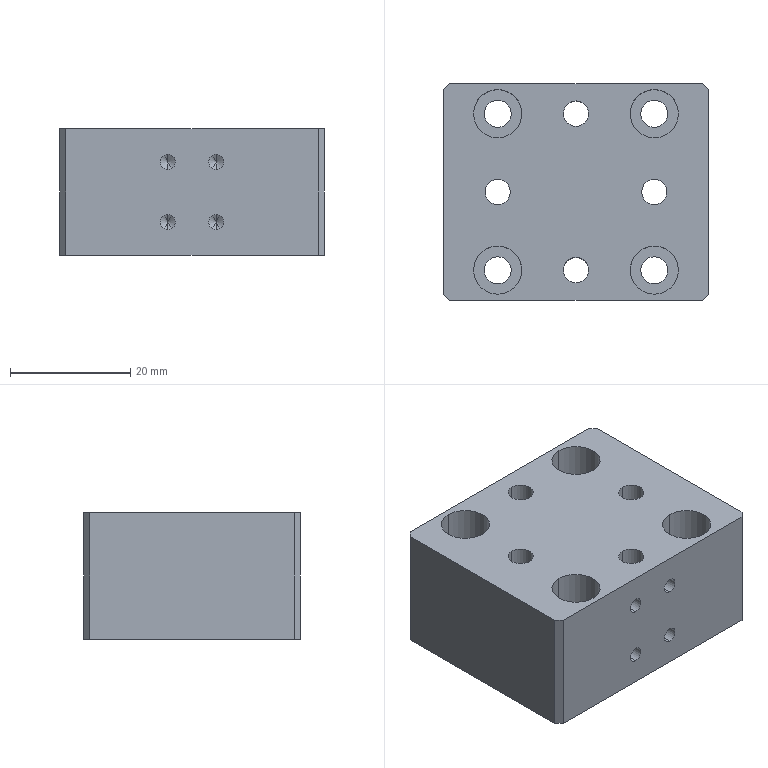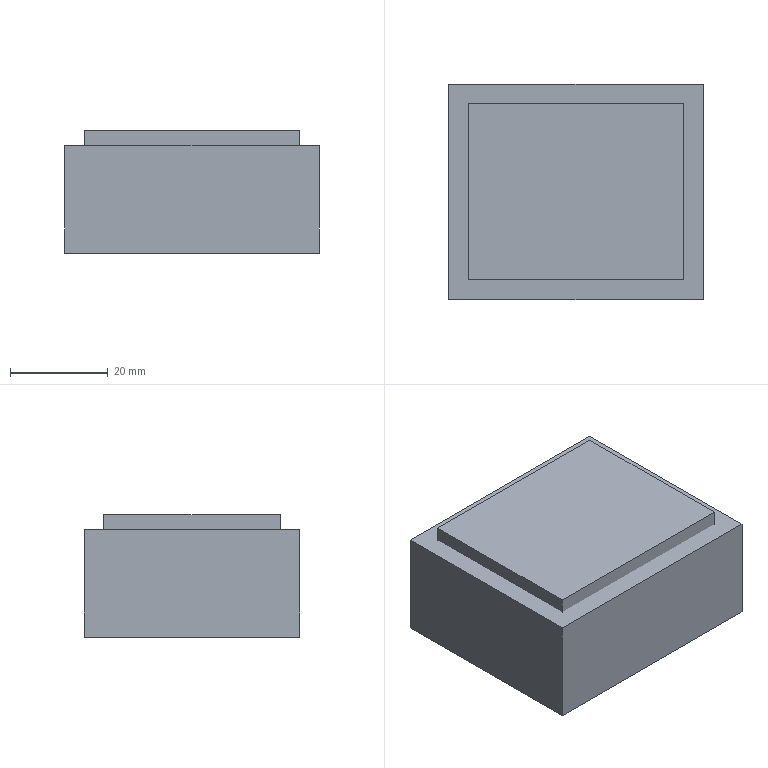CAM job | NX | 3+2 milling, drilling | part box 44 x 36 x 21 mm | stock box 52 x 44 x 25 mm
Tools:
number,name,description,diameter,corner_radius,flute_length,length,flutes
1,D63,Milling Tool-5 Parameters,63.0,0.0,50.0,75.0,2
7,D6A45,Milling Tool-5 Parameters,6.0,0.0,3.0,3.0,2
14,4.2ZT,Drilling Tool,4.2,0.0,35.0,50.0,2
15,M5,Milling Tool-5 Parameters,4.2,0.0,30.0,30.0,4
16,4.5ZT,Drilling Tool,4.5,0.0,35.0,50.0,2
4,D4,Milling Tool-5 Parameters,4.0,0.0,50.0,75.0,2
10,D10,Milling Tool-5 Parameters,10.0,0.0,50.0,75.0,2
11,D10JING,Milling Tool-5 Parameters,10.0,0.0,50.0,75.0,2
12,2.5ZT,Drilling Tool,2.5,0.0,35.0,50.0,2
13,M3,Milling Tool-5 Parameters,2.5,0.0,30.0,30.0,4
Operations:
program,operation,operation_type,tool,method,geometry_group,spindle_rpm,surface_speed,feed_per_tooth,feed_cut,feed_plunge,cut_length_mm,path_length_mm,cut_time_min,machine_time_min
1,FLOOR_WALL,VolumeBased25DMillingOperation,D63,METHOD,A,6500.0,1286.0,0.0962,1250.0,100.0,127.0,181.0,0.1016,0.107
1,DRILLING_COPY_1,Operation,D6A45,METHOD,A,5000.0,94.0,0.025,250.0,0.0,44.8,263.992,0.1792,0.2011
1,DRILLING_COPY,Operation,4.2ZT,METHOD,A,2000.0,39.0,0.0375,150.0,0.0,107.047,338.978,0.7136,0.7368
1,DRILLING_COPY_COPY,Operation,M5,METHOD,A,200.0,2.0,0.001,0.8,0.0,98.0,320.884,122.5,122.522
1,DRILLING_COPY_COPY_1,Operation,4.5ZT,METHOD,A,2000.0,39.0,0.0375,150.0,0.0,107.408,362.333,0.7161,0.7415
1,HOLE_MILLING,CylinderMilling,D4,METHOD,A,9500.0,119.0,0.0737,1400.0,100.0,1618.537,1994.537,1.156,1.194
1,HOLE_MILLING_COPY,CylinderMilling,D4,METHOD,A,9500.0,119.0,0.0737,1400.0,100.0,469.859,845.859,0.3356,0.3732
1,ADAPTIVE_MILLING,CavityMilling,D10,METHOD,A,9500.0,298.0,0.1579,3000.0,1000.0,1189.301,1287.301,0.3971,0.4069
1,ZLEVEL_PROFILE_COPY_COPY_1,ZLevelMilling,D10JING,METHOD,A,9500.0,298.0,0.0632,1200.0,100.0,197.093,293.093,0.1642,0.1738
1,ZLEVEL_PROFILE_1_COPY_1,ZLevelMilling,D6A45,METHOD,A,9500.0,179.0,0.0526,1000.0,100.0,316.155,1047.317,0.3162,0.3893
2,FLOOR_WALL_COPY,VolumeBased25DMillingOperation,D63,METHOD,B,6500.0,1286.0,0.0962,1250.0,100.0,476.0,1019.001,0.3808,0.4351
2,ZLEVEL_PROFILE_1_COPY_1_COPY,ZLevelMilling,D6A45,METHOD,B,9500.0,179.0,0.0526,1000.0,100.0,265.685,996.127,0.2657,0.3387
3,DRILLING_COPY_1_COPY,Operation,D6A45,METHOD,C,5000.0,94.0,0.025,250.0,0.0,18.4,142.546,0.0736,0.086
3,DRILLING_COPY_COPY_2,Operation,2.5ZT,METHOD,C,2000.0,39.0,0.0375,150.0,0.0,45.004,195.755,0.3,0.3151
3,DRILLING_COPY_COPY_2_COPY,Operation,M3,METHOD,C,200.0,1.0,0.0006,0.5,0.0,42.0,189.746,84.0,84.015